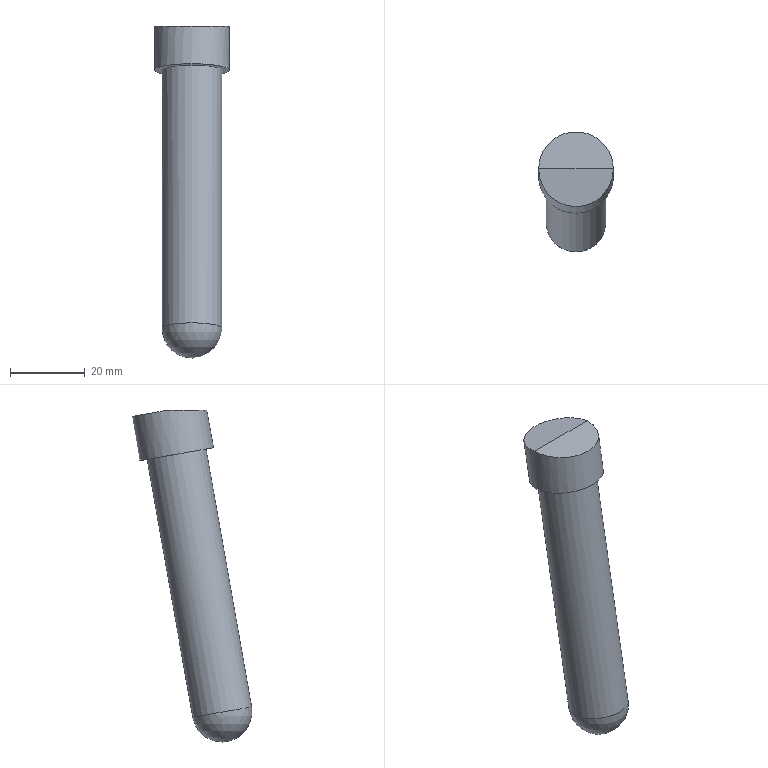Part | STEP file | P011002S004-008 | 1 solid | 6 faces | box 20 x 32.087 x 88.754 mm | volume 18799 mm3 | plane 3 | cylinder 2 | sphere 1 | commonest cylinder face diameters 16 x1 20 x1
STEP:
#1=CARTESIAN_POINT('',(0.,0.,0.));
#2=DIRECTION('',(0.,0.,1.));
#3=DIRECTION('',(1.,0.,0.));
#4=AXIS2_PLACEMENT_3D('',#1,#2,#3);
#5=CARTESIAN_POINT('',(25.,-220.,91.));
#6=VERTEX_POINT('',#5);
#7=CARTESIAN_POINT('',(45.,-220.,91.));
#8=VERTEX_POINT('',#7);
#9=CARTESIAN_POINT('',(35.,-220.,91.));
#10=DIRECTION('',(1.,0.,0.));
#11=VECTOR('',#10,1.);
#12=LINE('',#9,#11);
#13=CARTESIAN_POINT('',(35.,-220.,91.));
#14=DIRECTION('',(0.,-0.1736,-0.9848));
#15=DIRECTION('',(0.,0.9848,-0.1736));
#16=AXIS2_PLACEMENT_3D('',#13,#14,#15);
#17=PLANE('',#16);
#18=CARTESIAN_POINT('',(0.,0.));
#19=DIRECTION('',(0.,1.));
#20=VECTOR('',#19,1.);
#21=LINE('',#18,#20);
#22=(GEOMETRIC_REPRESENTATION_CONTEXT(2)PARAMETRIC_REPRESENTATION_CONTEXT()REPRESENTATION_CONTEXT('',''));
#23=DEFINITIONAL_REPRESENTATION('',(#21),#22);
#24=PCURVE('',#17,#23);
#25=CARTESIAN_POINT('',(2.5,-285.,91.));
#26=DIRECTION('',(0.,0.,1.));
#27=DIRECTION('',(-1.,0.,0.));
#28=AXIS2_PLACEMENT_3D('',#25,#26,#27);
#29=PLANE('',#28);
#30=CARTESIAN_POINT('',(-32.5,-65.));
#31=DIRECTION('',(-1.,0.));
#32=VECTOR('',#31,1.);
#33=LINE('',#30,#32);
#34=(GEOMETRIC_REPRESENTATION_CONTEXT(2)PARAMETRIC_REPRESENTATION_CONTEXT()REPRESENTATION_CONTEXT('',''));
#35=DEFINITIONAL_REPRESENTATION('',(#33),#34);
#36=PCURVE('',#29,#35);
#37=SURFACE_CURVE('',#12,(#24,#36),.PCURVE_S1.);
#38=EDGE_CURVE('',#6,#8,#37,.T.);
#39=ORIENTED_EDGE('',*,*,#38,.T.);
#40=CARTESIAN_POINT('',(35.,-220.,91.));
#41=DIRECTION('',(0.,0.1736,0.9848));
#42=DIRECTION('',(0.,0.9848,-0.1736));
#43=AXIS2_PLACEMENT_3D('',#40,#41,#42);
#44=CIRCLE('',#43,10.);
#45=CARTESIAN_POINT('',(10.,0.));
#46=CARTESIAN_POINT('',(10.,-17.321));
#47=CARTESIAN_POINT('',(-5.,-8.66));
#48=CARTESIAN_POINT('',(-20.,0.));
#49=CARTESIAN_POINT('',(-5.,8.66));
#50=CARTESIAN_POINT('',(10.,17.321));
#51=CARTESIAN_POINT('',(10.,0.));
#52=(BOUNDED_CURVE()B_SPLINE_CURVE(2,(#45,#46,#47,#48,#49,#50,#51),.UNSPECIFIED.,.T.,.F.)B_SPLINE_CURVE_WITH_KNOTS((1,2,2,2,2,1),(-2.094,0.,2.094,4.189,6.283,8.378),.UNSPECIFIED.)CURVE()GEOMETRIC_REPRESENTATION_ITEM()RATIONAL_B_SPLINE_CURVE((1.,0.5,1.,0.5,1.,0.5,1.))REPRESENTATION_ITEM(''));
#53=(GEOMETRIC_REPRESENTATION_CONTEXT(2)PARAMETRIC_REPRESENTATION_CONTEXT()REPRESENTATION_CONTEXT('',''));
#54=DEFINITIONAL_REPRESENTATION('',(#52),#53);
#55=PCURVE('',#17,#54);
#56=CARTESIAN_POINT('',(35.,-247.268,-63.644));
#57=DIRECTION('',(0.,0.1736,0.9848));
#58=DIRECTION('',(0.,-0.9848,0.1736));
#59=AXIS2_PLACEMENT_3D('',#56,#57,#58);
#60=CYLINDRICAL_SURFACE('',#59,10.);
#61=CARTESIAN_POINT('',(-3.142,157.029));
#62=DIRECTION('',(1.,0.));
#63=VECTOR('',#62,1.);
#64=LINE('',#61,#63);
#65=(GEOMETRIC_REPRESENTATION_CONTEXT(2)PARAMETRIC_REPRESENTATION_CONTEXT()REPRESENTATION_CONTEXT('',''));
#66=DEFINITIONAL_REPRESENTATION('',(#64),#65);
#67=PCURVE('',#60,#66);
#68=SURFACE_CURVE('',#44,(#55,#67),.PCURVE_S1.);
#69=EDGE_CURVE('',#8,#6,#68,.T.);
#70=ORIENTED_EDGE('',*,*,#69,.T.);
#71=EDGE_LOOP('',(#39,#70));
#72=FACE_BOUND('',#71,.T.);
#73=ADVANCED_FACE('',(#72),#17,.F.);
#74=CARTESIAN_POINT('',(35.,-231.932,80.919));
#75=VERTEX_POINT('',#74);
#76=CARTESIAN_POINT('',(35.,-222.084,79.182));
#77=DIRECTION('',(0.,-0.1736,-0.9848));
#78=DIRECTION('',(0.,-0.9848,0.1736));
#79=AXIS2_PLACEMENT_3D('',#76,#77,#78);
#80=CIRCLE('',#79,10.);
#81=CARTESIAN_POINT('',(6.283,145.029));
#82=DIRECTION('',(-1.,0.));
#83=VECTOR('',#82,1.);
#84=LINE('',#81,#83);
#85=(GEOMETRIC_REPRESENTATION_CONTEXT(2)PARAMETRIC_REPRESENTATION_CONTEXT()REPRESENTATION_CONTEXT('',''));
#86=DEFINITIONAL_REPRESENTATION('',(#84),#85);
#87=PCURVE('',#60,#86);
#88=CARTESIAN_POINT('',(70.,-222.084,79.182));
#89=DIRECTION('',(0.,0.1736,0.9848));
#90=DIRECTION('',(0.,-0.9848,0.1736));
#91=AXIS2_PLACEMENT_3D('',#88,#89,#90);
#92=PLANE('',#91);
#93=CARTESIAN_POINT('',(10.,-35.));
#94=CARTESIAN_POINT('',(10.,-52.321));
#95=CARTESIAN_POINT('',(-5.,-43.66));
#96=CARTESIAN_POINT('',(-20.,-35.));
#97=CARTESIAN_POINT('',(-5.,-26.34));
#98=CARTESIAN_POINT('',(10.,-17.679));
#99=CARTESIAN_POINT('',(10.,-35.));
#100=(BOUNDED_CURVE()B_SPLINE_CURVE(2,(#93,#94,#95,#96,#97,#98,#99),.UNSPECIFIED.,.T.,.F.)B_SPLINE_CURVE_WITH_KNOTS((1,2,2,2,2,1),(-2.094,0.,2.094,4.189,6.283,8.378),.UNSPECIFIED.)CURVE()GEOMETRIC_REPRESENTATION_ITEM()RATIONAL_B_SPLINE_CURVE((1.,0.5,1.,0.5,1.,0.5,1.))REPRESENTATION_ITEM(''));
#101=(GEOMETRIC_REPRESENTATION_CONTEXT(2)PARAMETRIC_REPRESENTATION_CONTEXT()REPRESENTATION_CONTEXT('',''));
#102=DEFINITIONAL_REPRESENTATION('',(#100),#101);
#103=PCURVE('',#92,#102);
#104=SURFACE_CURVE('',#80,(#87,#103),.PCURVE_S1.);
#105=EDGE_CURVE('',#75,#75,#104,.T.);
#106=ORIENTED_EDGE('',*,*,#105,.F.);
#107=CARTESIAN_POINT('',(35.,-230.154,91.));
#108=VERTEX_POINT('',#107);
#109=CARTESIAN_POINT('',(35.,-231.932,80.919));
#110=CARTESIAN_POINT('',(35.,-230.154,91.));
#111=B_SPLINE_CURVE_WITH_KNOTS('',1,(#109,#110),.UNSPECIFIED.,.F.,.F.,(2,2),(145.029,155.266),.PIECEWISE_BEZIER_KNOTS.);
#112=CARTESIAN_POINT('',(6.283,0.));
#113=DIRECTION('',(0.,1.));
#114=VECTOR('',#113,1.);
#115=LINE('',#112,#114);
#116=(GEOMETRIC_REPRESENTATION_CONTEXT(2)PARAMETRIC_REPRESENTATION_CONTEXT()REPRESENTATION_CONTEXT('',''));
#117=DEFINITIONAL_REPRESENTATION('',(#115),#116);
#118=PCURVE('',#60,#117);
#119=CARTESIAN_POINT('',(0.,0.));
#120=DIRECTION('',(0.,1.));
#121=VECTOR('',#120,1.);
#122=LINE('',#119,#121);
#123=(GEOMETRIC_REPRESENTATION_CONTEXT(2)PARAMETRIC_REPRESENTATION_CONTEXT()REPRESENTATION_CONTEXT('',''));
#124=DEFINITIONAL_REPRESENTATION('',(#122),#123);
#125=PCURVE('',#60,#124);
#126=SEAM_CURVE('',#111,(#118,#125),.PCURVE_S1.);
#127=EDGE_CURVE('',#75,#108,#126,.T.);
#128=ORIENTED_EDGE('',*,*,#127,.T.);
#129=CARTESIAN_POINT('',(35.,-220.,91.));
#130=DIRECTION('',(0.,0.,-1.));
#131=DIRECTION('',(0.,1.,0.));
#132=AXIS2_PLACEMENT_3D('',#129,#130,#131);
#133=ELLIPSE('',#132,10.154,10.);
#134=CARTESIAN_POINT('',(7.854,157.029));
#135=CARTESIAN_POINT('',(7.806,156.945));
#136=CARTESIAN_POINT('',(7.711,156.777));
#137=CARTESIAN_POINT('',(7.568,156.531));
#138=CARTESIAN_POINT('',(7.426,156.294));
#139=CARTESIAN_POINT('',(7.283,156.073));
#140=CARTESIAN_POINT('',(7.14,155.871));
#141=CARTESIAN_POINT('',(6.997,155.692));
#142=CARTESIAN_POINT('',(6.854,155.541));
#143=CARTESIAN_POINT('',(6.712,155.42));
#144=CARTESIAN_POINT('',(6.569,155.332));
#145=CARTESIAN_POINT('',(6.426,155.278));
#146=CARTESIAN_POINT('',(6.283,155.26));
#147=CARTESIAN_POINT('',(6.14,155.278));
#148=CARTESIAN_POINT('',(5.998,155.332));
#149=CARTESIAN_POINT('',(5.855,155.42));
#150=CARTESIAN_POINT('',(5.712,155.541));
#151=CARTESIAN_POINT('',(5.569,155.692));
#152=CARTESIAN_POINT('',(5.426,155.871));
#153=CARTESIAN_POINT('',(5.284,156.073));
#154=CARTESIAN_POINT('',(5.141,156.294));
#155=CARTESIAN_POINT('',(4.998,156.531));
#156=CARTESIAN_POINT('',(4.855,156.777));
#157=CARTESIAN_POINT('',(4.76,156.945));
#158=CARTESIAN_POINT('',(4.712,157.029));
#159=B_SPLINE_CURVE_WITH_KNOTS('',3,(#134,#135,#136,#137,#138,#139,#140,#141,#142,#143,#144,#145,#146,#147,#148,#149,#150,#151,#152,#153,#154,#155,#156,#157,#158),.UNSPECIFIED.,.F.,.F.,(4,1,1,1,1,1,1,1,1,1,1,1,1,1,1,1,1,1,1,1,1,1,4),(1.571,1.714,1.856,1.999,2.142,2.285,2.428,2.57,2.713,2.856,2.999,3.142,3.284,3.427,3.57,3.713,3.856,3.998,4.141,4.284,4.427,4.57,4.712),.QUASI_UNIFORM_KNOTS.);
#160=(GEOMETRIC_REPRESENTATION_CONTEXT(2)PARAMETRIC_REPRESENTATION_CONTEXT()REPRESENTATION_CONTEXT('',''));
#161=DEFINITIONAL_REPRESENTATION('',(#159),#160);
#162=PCURVE('',#60,#161);
#163=CARTESIAN_POINT('',(-32.5,-75.154));
#164=CARTESIAN_POINT('',(-49.821,-75.154));
#165=CARTESIAN_POINT('',(-41.16,-59.923));
#166=CARTESIAN_POINT('',(-32.5,-44.691));
#167=CARTESIAN_POINT('',(-23.84,-59.923));
#168=CARTESIAN_POINT('',(-15.179,-75.154));
#169=CARTESIAN_POINT('',(-32.5,-75.154));
#170=(BOUNDED_CURVE()B_SPLINE_CURVE(2,(#163,#164,#165,#166,#167,#168,#169),.UNSPECIFIED.,.T.,.F.)B_SPLINE_CURVE_WITH_KNOTS((1,2,2,2,2,1),(-2.094,0.,2.094,4.189,6.283,8.378),.UNSPECIFIED.)CURVE()GEOMETRIC_REPRESENTATION_ITEM()RATIONAL_B_SPLINE_CURVE((1.,0.5,1.,0.5,1.,0.5,1.))REPRESENTATION_ITEM(''));
#171=(GEOMETRIC_REPRESENTATION_CONTEXT(2)PARAMETRIC_REPRESENTATION_CONTEXT()REPRESENTATION_CONTEXT('',''));
#172=DEFINITIONAL_REPRESENTATION('',(#170),#171);
#173=PCURVE('',#29,#172);
#174=SURFACE_CURVE('',#133,(#162,#173),.PCURVE_S1.);
#175=EDGE_CURVE('',#108,#6,#174,.T.);
#176=ORIENTED_EDGE('',*,*,#175,.T.);
#177=ORIENTED_EDGE('',*,*,#69,.F.);
#178=CARTESIAN_POINT('',(35.,-220.,91.));
#179=DIRECTION('',(0.,0.,-1.));
#180=DIRECTION('',(0.,1.,0.));
#181=AXIS2_PLACEMENT_3D('',#178,#179,#180);
#182=ELLIPSE('',#181,10.154,10.);
#183=CARTESIAN_POINT('',(1.571,157.029));
#184=CARTESIAN_POINT('',(1.523,156.945));
#185=CARTESIAN_POINT('',(1.428,156.777));
#186=CARTESIAN_POINT('',(1.285,156.531));
#187=CARTESIAN_POINT('',(1.142,156.294));
#188=CARTESIAN_POINT('',(0.9996,156.073));
#189=CARTESIAN_POINT('',(0.8568,155.871));
#190=CARTESIAN_POINT('',(0.714,155.692));
#191=CARTESIAN_POINT('',(0.5712,155.541));
#192=CARTESIAN_POINT('',(0.4284,155.42));
#193=CARTESIAN_POINT('',(0.2856,155.332));
#194=CARTESIAN_POINT('',(0.1428,155.278));
#195=CARTESIAN_POINT('',(0.,155.26));
#196=CARTESIAN_POINT('',(-0.1428,155.278));
#197=CARTESIAN_POINT('',(-0.2856,155.332));
#198=CARTESIAN_POINT('',(-0.4284,155.42));
#199=CARTESIAN_POINT('',(-0.5712,155.541));
#200=CARTESIAN_POINT('',(-0.714,155.692));
#201=CARTESIAN_POINT('',(-0.8568,155.871));
#202=CARTESIAN_POINT('',(-0.9996,156.073));
#203=CARTESIAN_POINT('',(-1.142,156.294));
#204=CARTESIAN_POINT('',(-1.285,156.531));
#205=CARTESIAN_POINT('',(-1.428,156.777));
#206=CARTESIAN_POINT('',(-1.523,156.945));
#207=CARTESIAN_POINT('',(-1.571,157.029));
#208=B_SPLINE_CURVE_WITH_KNOTS('',3,(#183,#184,#185,#186,#187,#188,#189,#190,#191,#192,#193,#194,#195,#196,#197,#198,#199,#200,#201,#202,#203,#204,#205,#206,#207),.UNSPECIFIED.,.F.,.F.,(4,1,1,1,1,1,1,1,1,1,1,1,1,1,1,1,1,1,1,1,1,1,4),(1.571,1.714,1.856,1.999,2.142,2.285,2.428,2.57,2.713,2.856,2.999,3.142,3.284,3.427,3.57,3.713,3.856,3.998,4.141,4.284,4.427,4.57,4.712),.QUASI_UNIFORM_KNOTS.);
#209=(GEOMETRIC_REPRESENTATION_CONTEXT(2)PARAMETRIC_REPRESENTATION_CONTEXT()REPRESENTATION_CONTEXT('',''));
#210=DEFINITIONAL_REPRESENTATION('',(#208),#209);
#211=PCURVE('',#60,#210);
#212=CARTESIAN_POINT('',(-32.5,-75.154));
#213=CARTESIAN_POINT('',(-49.821,-75.154));
#214=CARTESIAN_POINT('',(-41.16,-59.923));
#215=CARTESIAN_POINT('',(-32.5,-44.691));
#216=CARTESIAN_POINT('',(-23.84,-59.923));
#217=CARTESIAN_POINT('',(-15.179,-75.154));
#218=CARTESIAN_POINT('',(-32.5,-75.154));
#219=(BOUNDED_CURVE()B_SPLINE_CURVE(2,(#212,#213,#214,#215,#216,#217,#218),.UNSPECIFIED.,.T.,.F.)B_SPLINE_CURVE_WITH_KNOTS((1,2,2,2,2,1),(-2.094,0.,2.094,4.189,6.283,8.378),.UNSPECIFIED.)CURVE()GEOMETRIC_REPRESENTATION_ITEM()RATIONAL_B_SPLINE_CURVE((1.,0.5,1.,0.5,1.,0.5,1.))REPRESENTATION_ITEM(''));
#220=(GEOMETRIC_REPRESENTATION_CONTEXT(2)PARAMETRIC_REPRESENTATION_CONTEXT()REPRESENTATION_CONTEXT('',''));
#221=DEFINITIONAL_REPRESENTATION('',(#219),#220);
#222=PCURVE('',#29,#221);
#223=SURFACE_CURVE('',#182,(#211,#222),.PCURVE_S1.);
#224=EDGE_CURVE('',#8,#108,#223,.T.);
#225=ORIENTED_EDGE('',*,*,#224,.T.);
#226=ORIENTED_EDGE('',*,*,#127,.F.);
#227=EDGE_LOOP('',(#106,#128,#176,#177,#225,#226));
#228=FACE_BOUND('',#227,.T.);
#229=ADVANCED_FACE('',(#228),#60,.T.);
#230=CARTESIAN_POINT('',(35.,-242.118,11.635));
#231=VERTEX_POINT('',#230);
#232=CARTESIAN_POINT('',(27.,-234.239,10.246));
#233=VERTEX_POINT('',#232);
#234=CARTESIAN_POINT('',(35.,-234.239,10.246));
#235=DIRECTION('',(0.,-0.1736,-0.9848));
#236=DIRECTION('',(0.,-0.9848,0.1736));
#237=AXIS2_PLACEMENT_3D('',#234,#235,#236);
#238=CIRCLE('',#237,8.);
#239=CARTESIAN_POINT('',(35.,-247.268,-63.644));
#240=DIRECTION('',(0.,0.1736,0.9848));
#241=DIRECTION('',(0.,-0.9848,0.1736));
#242=AXIS2_PLACEMENT_3D('',#239,#240,#241);
#243=CYLINDRICAL_SURFACE('',#242,8.);
#244=CARTESIAN_POINT('',(6.283,75.029));
#245=DIRECTION('',(-1.,0.));
#246=VECTOR('',#245,1.);
#247=LINE('',#244,#246);
#248=(GEOMETRIC_REPRESENTATION_CONTEXT(2)PARAMETRIC_REPRESENTATION_CONTEXT()REPRESENTATION_CONTEXT('',''));
#249=DEFINITIONAL_REPRESENTATION('',(#247),#248);
#250=PCURVE('',#243,#249);
#251=CARTESIAN_POINT('',(35.,-234.239,10.246));
#252=DIRECTION('',(0.,0.,1.));
#253=DIRECTION('',(-1.,0.,0.));
#254=AXIS2_PLACEMENT_3D('',#251,#252,#253);
#255=SPHERICAL_SURFACE('',#254,8.);
#256=CARTESIAN_POINT('',(1.571,0.1745));
#257=CARTESIAN_POINT('',(1.474,0.1746));
#258=CARTESIAN_POINT('',(1.281,0.1697));
#259=CARTESIAN_POINT('',(0.9922,0.1486));
#260=CARTESIAN_POINT('',(0.706,0.1155));
#261=CARTESIAN_POINT('',(0.4223,0.07316));
#262=CARTESIAN_POINT('',(0.1405,0.02504));
#263=CARTESIAN_POINT('',(-0.1405,-0.02504));
#264=CARTESIAN_POINT('',(-0.4223,-0.07316));
#265=CARTESIAN_POINT('',(-0.706,-0.1155));
#266=CARTESIAN_POINT('',(-0.9922,-0.1486));
#267=CARTESIAN_POINT('',(-1.281,-0.1697));
#268=CARTESIAN_POINT('',(-1.571,-0.1769));
#269=CARTESIAN_POINT('',(-1.861,-0.1697));
#270=CARTESIAN_POINT('',(-2.149,-0.1486));
#271=CARTESIAN_POINT('',(-2.436,-0.1155));
#272=CARTESIAN_POINT('',(-2.719,-0.07316));
#273=CARTESIAN_POINT('',(-3.001,-0.02504));
#274=CARTESIAN_POINT('',(-3.282,0.02504));
#275=CARTESIAN_POINT('',(-3.564,0.07316));
#276=CARTESIAN_POINT('',(-3.848,0.1155));
#277=CARTESIAN_POINT('',(-4.134,0.1486));
#278=CARTESIAN_POINT('',(-4.422,0.1697));
#279=CARTESIAN_POINT('',(-4.616,0.1746));
#280=CARTESIAN_POINT('',(-4.712,0.1745));
#281=B_SPLINE_CURVE_WITH_KNOTS('',3,(#256,#257,#258,#259,#260,#261,#262,#263,#264,#265,#266,#267,#268,#269,#270,#271,#272,#273,#274,#275,#276,#277,#278,#279,#280),.UNSPECIFIED.,.F.,.F.,(4,1,1,1,1,1,1,1,1,1,1,1,1,1,1,1,1,1,1,1,1,1,4),(0.,0.2856,0.5712,0.8568,1.142,1.428,1.714,1.999,2.285,2.57,2.856,3.142,3.427,3.713,3.998,4.284,4.57,4.855,5.141,5.426,5.712,5.998,6.283),.QUASI_UNIFORM_KNOTS.);
#282=(GEOMETRIC_REPRESENTATION_CONTEXT(2)PARAMETRIC_REPRESENTATION_CONTEXT()REPRESENTATION_CONTEXT('',''));
#283=DEFINITIONAL_REPRESENTATION('',(#281),#282);
#284=PCURVE('',#255,#283);
#285=SURFACE_CURVE('',#238,(#250,#284),.PCURVE_S1.);
#286=EDGE_CURVE('',#231,#233,#285,.T.);
#287=ORIENTED_EDGE('',*,*,#286,.F.);
#288=CARTESIAN_POINT('',(35.,-229.962,80.571));
#289=VERTEX_POINT('',#288);
#290=CARTESIAN_POINT('',(35.,-242.118,11.635));
#291=CARTESIAN_POINT('',(35.,-229.962,80.571));
#292=B_SPLINE_CURVE_WITH_KNOTS('',1,(#290,#291),.UNSPECIFIED.,.F.,.F.,(2,2),(75.029,145.029),.PIECEWISE_BEZIER_KNOTS.);
#293=CARTESIAN_POINT('',(6.283,0.));
#294=DIRECTION('',(0.,1.));
#295=VECTOR('',#294,1.);
#296=LINE('',#293,#295);
#297=(GEOMETRIC_REPRESENTATION_CONTEXT(2)PARAMETRIC_REPRESENTATION_CONTEXT()REPRESENTATION_CONTEXT('',''));
#298=DEFINITIONAL_REPRESENTATION('',(#296),#297);
#299=PCURVE('',#243,#298);
#300=CARTESIAN_POINT('',(0.,0.));
#301=DIRECTION('',(0.,1.));
#302=VECTOR('',#301,1.);
#303=LINE('',#300,#302);
#304=(GEOMETRIC_REPRESENTATION_CONTEXT(2)PARAMETRIC_REPRESENTATION_CONTEXT()REPRESENTATION_CONTEXT('',''));
#305=DEFINITIONAL_REPRESENTATION('',(#303),#304);
#306=PCURVE('',#243,#305);
#307=SEAM_CURVE('',#292,(#299,#306),.PCURVE_S1.);
#308=EDGE_CURVE('',#231,#289,#307,.T.);
#309=ORIENTED_EDGE('',*,*,#308,.T.);
#310=CARTESIAN_POINT('',(35.,-222.084,79.182));
#311=DIRECTION('',(0.,-0.1736,-0.9848));
#312=DIRECTION('',(0.,-0.9848,0.1736));
#313=AXIS2_PLACEMENT_3D('',#310,#311,#312);
#314=CIRCLE('',#313,8.);
#315=CARTESIAN_POINT('',(6.283,145.029));
#316=DIRECTION('',(-1.,0.));
#317=VECTOR('',#316,1.);
#318=LINE('',#315,#317);
#319=(GEOMETRIC_REPRESENTATION_CONTEXT(2)PARAMETRIC_REPRESENTATION_CONTEXT()REPRESENTATION_CONTEXT('',''));
#320=DEFINITIONAL_REPRESENTATION('',(#318),#319);
#321=PCURVE('',#243,#320);
#322=CARTESIAN_POINT('',(8.,-35.));
#323=CARTESIAN_POINT('',(8.,-48.856));
#324=CARTESIAN_POINT('',(-4.,-41.928));
#325=CARTESIAN_POINT('',(-16.,-35.));
#326=CARTESIAN_POINT('',(-4.,-28.072));
#327=CARTESIAN_POINT('',(8.,-21.144));
#328=CARTESIAN_POINT('',(8.,-35.));
#329=(BOUNDED_CURVE()B_SPLINE_CURVE(2,(#322,#323,#324,#325,#326,#327,#328),.UNSPECIFIED.,.T.,.F.)B_SPLINE_CURVE_WITH_KNOTS((1,2,2,2,2,1),(-2.094,0.,2.094,4.189,6.283,8.378),.UNSPECIFIED.)CURVE()GEOMETRIC_REPRESENTATION_ITEM()RATIONAL_B_SPLINE_CURVE((1.,0.5,1.,0.5,1.,0.5,1.))REPRESENTATION_ITEM(''));
#330=(GEOMETRIC_REPRESENTATION_CONTEXT(2)PARAMETRIC_REPRESENTATION_CONTEXT()REPRESENTATION_CONTEXT('',''));
#331=DEFINITIONAL_REPRESENTATION('',(#329),#330);
#332=PCURVE('',#92,#331);
#333=SURFACE_CURVE('',#314,(#321,#332),.PCURVE_S1.);
#334=EDGE_CURVE('',#289,#289,#333,.T.);
#335=ORIENTED_EDGE('',*,*,#334,.T.);
#336=ORIENTED_EDGE('',*,*,#308,.F.);
#337=CARTESIAN_POINT('',(35.,-234.239,10.246));
#338=DIRECTION('',(0.,-0.1736,-0.9848));
#339=DIRECTION('',(0.,-0.9848,0.1736));
#340=AXIS2_PLACEMENT_3D('',#337,#338,#339);
#341=CIRCLE('',#340,8.);
#342=CARTESIAN_POINT('',(6.283,75.029));
#343=DIRECTION('',(-1.,0.));
#344=VECTOR('',#343,1.);
#345=LINE('',#342,#344);
#346=(GEOMETRIC_REPRESENTATION_CONTEXT(2)PARAMETRIC_REPRESENTATION_CONTEXT()REPRESENTATION_CONTEXT('',''));
#347=DEFINITIONAL_REPRESENTATION('',(#345),#346);
#348=PCURVE('',#243,#347);
#349=CARTESIAN_POINT('',(7.854,0.1745));
#350=CARTESIAN_POINT('',(7.757,0.1746));
#351=CARTESIAN_POINT('',(7.564,0.1697));
#352=CARTESIAN_POINT('',(7.275,0.1486));
#353=CARTESIAN_POINT('',(6.989,0.1155));
#354=CARTESIAN_POINT('',(6.706,0.07316));
#355=CARTESIAN_POINT('',(6.424,0.02504));
#356=CARTESIAN_POINT('',(6.143,-0.02504));
#357=CARTESIAN_POINT('',(5.861,-0.07316));
#358=CARTESIAN_POINT('',(5.577,-0.1155));
#359=CARTESIAN_POINT('',(5.291,-0.1486));
#360=CARTESIAN_POINT('',(5.002,-0.1697));
#361=CARTESIAN_POINT('',(4.712,-0.1769));
#362=CARTESIAN_POINT('',(4.422,-0.1697));
#363=CARTESIAN_POINT('',(4.134,-0.1486));
#364=CARTESIAN_POINT('',(3.848,-0.1155));
#365=CARTESIAN_POINT('',(3.564,-0.07316));
#366=CARTESIAN_POINT('',(3.282,-0.02504));
#367=CARTESIAN_POINT('',(3.001,0.02504));
#368=CARTESIAN_POINT('',(2.719,0.07316));
#369=CARTESIAN_POINT('',(2.436,0.1155));
#370=CARTESIAN_POINT('',(2.149,0.1486));
#371=CARTESIAN_POINT('',(1.861,0.1697));
#372=CARTESIAN_POINT('',(1.668,0.1746));
#373=CARTESIAN_POINT('',(1.571,0.1745));
#374=B_SPLINE_CURVE_WITH_KNOTS('',3,(#349,#350,#351,#352,#353,#354,#355,#356,#357,#358,#359,#360,#361,#362,#363,#364,#365,#366,#367,#368,#369,#370,#371,#372,#373),.UNSPECIFIED.,.F.,.F.,(4,1,1,1,1,1,1,1,1,1,1,1,1,1,1,1,1,1,1,1,1,1,4),(0.,0.2856,0.5712,0.8568,1.142,1.428,1.714,1.999,2.285,2.57,2.856,3.142,3.427,3.713,3.998,4.284,4.57,4.855,5.141,5.426,5.712,5.998,6.283),.QUASI_UNIFORM_KNOTS.);
#375=(GEOMETRIC_REPRESENTATION_CONTEXT(2)PARAMETRIC_REPRESENTATION_CONTEXT()REPRESENTATION_CONTEXT('',''));
#376=DEFINITIONAL_REPRESENTATION('',(#374),#375);
#377=PCURVE('',#255,#376);
#378=SURFACE_CURVE('',#341,(#348,#377),.PCURVE_S1.);
#379=EDGE_CURVE('',#233,#231,#378,.T.);
#380=ORIENTED_EDGE('',*,*,#379,.F.);
#381=EDGE_LOOP('',(#287,#309,#335,#336,#380));
#382=FACE_BOUND('',#381,.T.);
#383=ADVANCED_FACE('',(#382),#243,.T.);
#384=ORIENTED_EDGE('',*,*,#105,.T.);
#385=EDGE_LOOP('',(#384));
#386=FACE_BOUND('',#385,.T.);
#387=ORIENTED_EDGE('',*,*,#334,.F.);
#388=EDGE_LOOP('',(#387));
#389=FACE_BOUND('',#388,.T.);
#390=ADVANCED_FACE('',(#386,#389),#92,.F.);
#391=ORIENTED_EDGE('',*,*,#286,.T.);
#392=CARTESIAN_POINT('',(35.,-234.239,2.246));
#393=VERTEX_POINT('',#392);
#394=CARTESIAN_POINT('',(35.,-234.239,2.246));
#395=CARTESIAN_POINT('',(33.205,-234.239,2.246));
#396=CARTESIAN_POINT('',(31.41,-234.239,2.716));
#397=CARTESIAN_POINT('',(29.762,-234.239,3.656));
#398=CARTESIAN_POINT('',(28.41,-234.239,5.008));
#399=CARTESIAN_POINT('',(27.47,-234.239,6.655));
#400=CARTESIAN_POINT('',(27.,-234.239,8.451));
#401=CARTESIAN_POINT('',(27.,-234.239,10.246));
#402=B_SPLINE_CURVE_WITH_KNOTS('',7,(#394,#395,#396,#397,#398,#399,#400,#401),.UNSPECIFIED.,.F.,.F.,(8,8),(-1.571,-0.000000068),.PIECEWISE_BEZIER_KNOTS.);
#403=CARTESIAN_POINT('',(0.,0.));
#404=DIRECTION('',(0.,1.));
#405=VECTOR('',#404,1.);
#406=LINE('',#403,#405);
#407=(GEOMETRIC_REPRESENTATION_CONTEXT(2)PARAMETRIC_REPRESENTATION_CONTEXT()REPRESENTATION_CONTEXT('',''));
#408=DEFINITIONAL_REPRESENTATION('',(#406),#407);
#409=PCURVE('',#255,#408);
#410=CARTESIAN_POINT('',(6.283,0.));
#411=DIRECTION('',(0.,1.));
#412=VECTOR('',#411,1.);
#413=LINE('',#410,#412);
#414=(GEOMETRIC_REPRESENTATION_CONTEXT(2)PARAMETRIC_REPRESENTATION_CONTEXT()REPRESENTATION_CONTEXT('',''));
#415=DEFINITIONAL_REPRESENTATION('',(#413),#414);
#416=PCURVE('',#255,#415);
#417=SEAM_CURVE('',#402,(#409,#416),.PCURVE_S1.);
#418=EDGE_CURVE('',#393,#233,#417,.T.);
#419=ORIENTED_EDGE('',*,*,#418,.F.);
#420=ORIENTED_EDGE('',*,*,#418,.T.);
#421=ORIENTED_EDGE('',*,*,#379,.T.);
#422=EDGE_LOOP('',(#391,#419,#420,#421));
#423=FACE_BOUND('',#422,.T.);
#424=ADVANCED_FACE('',(#423),#255,.T.);
#425=ORIENTED_EDGE('',*,*,#224,.F.);
#426=ORIENTED_EDGE('',*,*,#38,.F.);
#427=ORIENTED_EDGE('',*,*,#175,.F.);
#428=EDGE_LOOP('',(#425,#426,#427));
#429=FACE_BOUND('',#428,.T.);
#430=ADVANCED_FACE('',(#429),#29,.T.);
#431=CLOSED_SHELL('',(#73,#229,#383,#390,#424,#430));
#432=MANIFOLD_SOLID_BREP('',#431);
#433=(LENGTH_UNIT()NAMED_UNIT(*)SI_UNIT(.MILLI.,.METRE.));
#434=UNCERTAINTY_MEASURE_WITH_UNIT(LENGTH_MEASURE(0.0001),#433,'','');
#435=(NAMED_UNIT(*)PLANE_ANGLE_UNIT()SI_UNIT($,.RADIAN.));
#436=(NAMED_UNIT(*)SI_UNIT($,.STERADIAN.)SOLID_ANGLE_UNIT());
#437=(GEOMETRIC_REPRESENTATION_CONTEXT(3)GLOBAL_UNCERTAINTY_ASSIGNED_CONTEXT((#434))GLOBAL_UNIT_ASSIGNED_CONTEXT((#433,#435,#436))REPRESENTATION_CONTEXT('',''));
#438=ADVANCED_BREP_SHAPE_REPRESENTATION('',(#4,#432),#437);